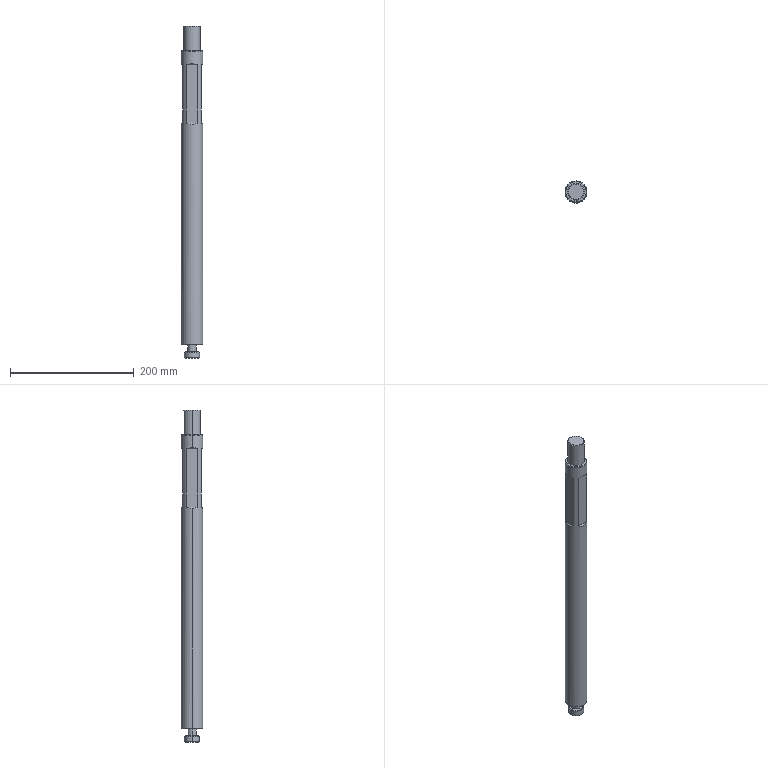Part | STEP file | Pino extrator para moldes PEQUENOS - SANDRETTO 450T - Torre - 1 cav | 1 solid | 35 faces | box 35 x 35 x 537.25 mm | volume 475534 mm3 | plane 17 | cone 10 | cylinder 8 | commonest cylinder face diameters 14 x2 24.5 x2 27 x2 35 x2